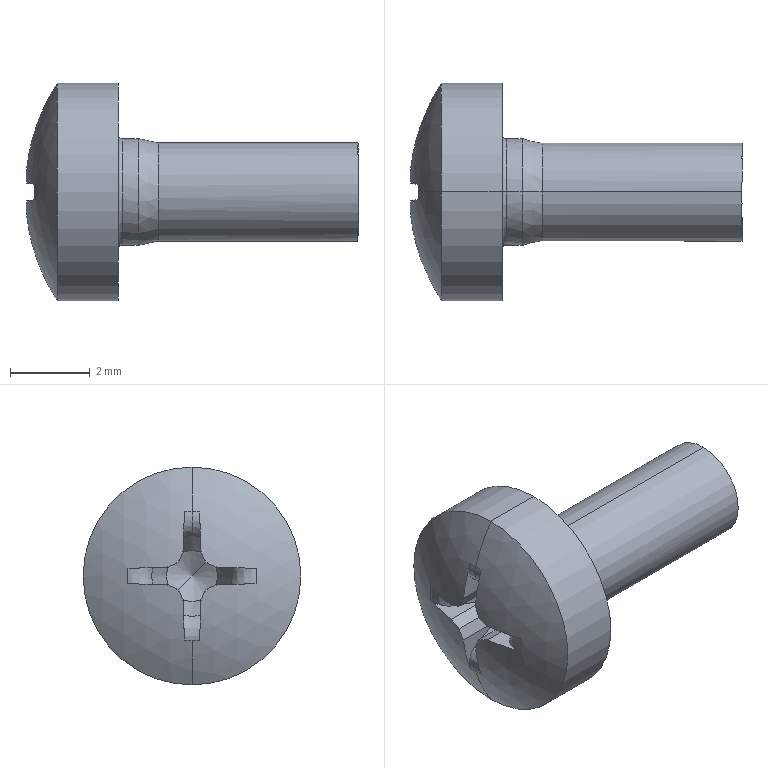Part | STEP file | 4-20.sldasm-Part-212 | 1 solid | 41 faces | box 8.306 x 5.45 x 5.45 mm | volume 72.235 mm3 | plane 18 | cone 8 | torus 7 | cylinder 6 | sphere 2 | commonest cylinder face diameters 2.458 x2 2.675 x2 5.45 x2
STEP:
#1=CARTESIAN_POINT('',(184.475,545.075,-91.754));
#2=VERTEX_POINT('',#1);
#3=CARTESIAN_POINT('',(184.475,545.075,-89.296));
#4=VERTEX_POINT('',#3);
#5=CARTESIAN_POINT('',(184.475,545.075,-90.525));
#6=DIRECTION('',(-1.,0.,0.));
#7=DIRECTION('',(0.,0.,1.));
#8=AXIS2_PLACEMENT_3D('',#5,#6,#7);
#9=CIRCLE('',#8,1.229);
#10=EDGE_CURVE('',#2,#4,#9,.T.);
#11=ORIENTED_EDGE('',*,*,#10,.T.);
#12=CARTESIAN_POINT('',(183.975,545.075,-89.188));
#13=VERTEX_POINT('',#12);
#14=CARTESIAN_POINT('',(184.475,545.075,-89.296));
#15=DIRECTION('',(-0.9776,0.,0.2107));
#16=VECTOR('',#15,1000.);
#17=LINE('',#14,#16);
#18=EDGE_CURVE('',#4,#13,#17,.T.);
#19=ORIENTED_EDGE('',*,*,#18,.T.);
#20=CARTESIAN_POINT('',(183.975,545.075,-91.862));
#21=VERTEX_POINT('',#20);
#22=CARTESIAN_POINT('',(183.975,545.075,-91.862));
#23=CARTESIAN_POINT('',(183.975,544.9,-91.863));
#24=CARTESIAN_POINT('',(183.975,544.725,-91.828));
#25=CARTESIAN_POINT('',(183.975,544.401,-91.694));
#26=CARTESIAN_POINT('',(183.975,544.253,-91.595));
#27=CARTESIAN_POINT('',(183.975,544.005,-91.347));
#28=CARTESIAN_POINT('',(183.975,543.906,-91.199));
#29=CARTESIAN_POINT('',(183.975,543.772,-90.875));
#30=CARTESIAN_POINT('',(183.975,543.737,-90.7));
#31=CARTESIAN_POINT('',(183.975,543.737,-90.35));
#32=CARTESIAN_POINT('',(183.975,543.772,-90.175));
#33=CARTESIAN_POINT('',(183.975,543.906,-89.851));
#34=CARTESIAN_POINT('',(183.975,544.005,-89.703));
#35=CARTESIAN_POINT('',(183.975,544.253,-89.455));
#36=CARTESIAN_POINT('',(183.975,544.401,-89.356));
#37=CARTESIAN_POINT('',(183.975,544.725,-89.222));
#38=CARTESIAN_POINT('',(183.975,544.9,-89.187));
#39=CARTESIAN_POINT('',(183.975,545.075,-89.188));
#40=B_SPLINE_CURVE_WITH_KNOTS('',3,(#22,#23,#24,#25,#26,#27,#28,#29,#30,#31,#32,#33,#34,#35,#36,#37,#38,#39),.UNSPECIFIED.,.F.,.F.,(4,2,2,2,2,2,2,2,4),(0.5,0.5625,0.625,0.6875,0.75,0.8125,0.875,0.9375,1.),.UNSPECIFIED.);
#41=EDGE_CURVE('',#21,#13,#40,.T.);
#42=ORIENTED_EDGE('',*,*,#41,.F.);
#43=CARTESIAN_POINT('',(184.475,545.075,-91.754));
#44=DIRECTION('',(-0.9776,0.,-0.2107));
#45=VECTOR('',#44,1000.);
#46=LINE('',#43,#45);
#47=EDGE_CURVE('',#2,#21,#46,.T.);
#48=ORIENTED_EDGE('',*,*,#47,.F.);
#49=EDGE_LOOP('',(#11,#19,#42,#48));
#50=FACE_OUTER_BOUND('',#49,.T.);
#51=CARTESIAN_POINT('',(184.475,545.075,-90.525));
#52=DIRECTION('',(-1.,0.,0.));
#53=DIRECTION('',(0.,0.,-1.));
#54=AXIS2_PLACEMENT_3D('',#51,#52,#53);
#55=CONICAL_SURFACE('',#54,1.229,0.2123);
#56=ADVANCED_FACE('',(#50),#55,.T.);
#57=ORIENTED_EDGE('',*,*,#10,.F.);
#58=CARTESIAN_POINT('',(189.475,545.075,-91.754));
#59=VERTEX_POINT('',#58);
#60=CARTESIAN_POINT('',(184.475,545.075,-91.754));
#61=DIRECTION('',(1.,0.,0.));
#62=VECTOR('',#61,1000.);
#63=LINE('',#60,#62);
#64=EDGE_CURVE('',#2,#59,#63,.T.);
#65=ORIENTED_EDGE('',*,*,#64,.T.);
#66=CARTESIAN_POINT('',(189.475,545.075,-89.296));
#67=VERTEX_POINT('',#66);
#68=CARTESIAN_POINT('',(189.475,545.075,-89.296));
#69=CARTESIAN_POINT('',(189.475,544.912,-89.296));
#70=CARTESIAN_POINT('',(189.475,544.756,-89.327));
#71=CARTESIAN_POINT('',(189.475,544.529,-89.421));
#72=CARTESIAN_POINT('',(189.475,544.423,-89.478));
#73=CARTESIAN_POINT('',(189.475,544.327,-89.549));
#74=CARTESIAN_POINT('',(189.475,544.265,-89.6));
#75=CARTESIAN_POINT('',(189.475,544.236,-89.626));
#76=CARTESIAN_POINT('',(189.475,543.966,-89.897));
#77=CARTESIAN_POINT('',(189.475,543.846,-90.185));
#78=CARTESIAN_POINT('',(189.475,543.846,-90.865));
#79=CARTESIAN_POINT('',(189.475,543.966,-91.154));
#80=CARTESIAN_POINT('',(189.475,544.447,-91.634));
#81=CARTESIAN_POINT('',(189.475,544.735,-91.754));
#82=CARTESIAN_POINT('',(189.475,545.075,-91.754));
#83=B_SPLINE_CURVE_WITH_KNOTS('',3,(#68,#69,#70,#71,#72,#73,#74,#75,#76,#77,#78,#79,#80,#81,#82),.UNSPECIFIED.,.F.,.F.,(4,2,1,2,2,2,2,4),(0.,0.0625,0.09375,0.1094,0.125,0.25,0.375,0.5),.UNSPECIFIED.);
#84=EDGE_CURVE('',#67,#59,#83,.T.);
#85=ORIENTED_EDGE('',*,*,#84,.F.);
#86=CARTESIAN_POINT('',(184.475,545.075,-89.296));
#87=DIRECTION('',(1.,0.,0.));
#88=VECTOR('',#87,1000.);
#89=LINE('',#86,#88);
#90=EDGE_CURVE('',#4,#67,#89,.T.);
#91=ORIENTED_EDGE('',*,*,#90,.F.);
#92=EDGE_LOOP('',(#57,#65,#85,#91));
#93=FACE_OUTER_BOUND('',#92,.T.);
#94=CARTESIAN_POINT('',(184.475,545.075,-90.525));
#95=DIRECTION('',(1.,0.,0.));
#96=DIRECTION('',(0.,0.,1.));
#97=AXIS2_PLACEMENT_3D('',#94,#95,#96);
#98=CYLINDRICAL_SURFACE('',#97,1.229);
#99=ADVANCED_FACE('',(#93),#98,.T.);
#100=CARTESIAN_POINT('',(181.663,545.281,-89.541));
#101=VERTEX_POINT('',#100);
#102=CARTESIAN_POINT('',(181.663,545.075,-89.52));
#103=VERTEX_POINT('',#102);
#104=CARTESIAN_POINT('',(181.663,545.075,-90.525));
#105=DIRECTION('',(1.,0.,0.));
#106=DIRECTION('',(0.,0.,-1.));
#107=AXIS2_PLACEMENT_3D('',#104,#105,#106);
#108=CIRCLE('',#107,1.005);
#109=EDGE_CURVE('',#101,#103,#108,.T.);
#110=ORIENTED_EDGE('',*,*,#109,.T.);
#111=CARTESIAN_POINT('',(181.413,545.075,-88.911));
#112=VERTEX_POINT('',#111);
#113=CARTESIAN_POINT('',(181.886,545.075,-89.072));
#114=DIRECTION('',(0.,1.,0.));
#115=DIRECTION('',(0.,0.,1.));
#116=AXIS2_PLACEMENT_3D('',#113,#114,#115);
#117=CIRCLE('',#116,0.5);
#118=EDGE_CURVE('',#103,#112,#117,.T.);
#119=ORIENTED_EDGE('',*,*,#118,.T.);
#120=CARTESIAN_POINT('',(181.413,545.27,-88.923));
#121=VERTEX_POINT('',#120);
#122=CARTESIAN_POINT('',(181.413,545.075,-90.525));
#123=DIRECTION('',(-1.,0.,0.));
#124=DIRECTION('',(0.,0.,1.));
#125=AXIS2_PLACEMENT_3D('',#122,#123,#124);
#126=CIRCLE('',#125,1.614);
#127=EDGE_CURVE('',#112,#121,#126,.T.);
#128=ORIENTED_EDGE('',*,*,#127,.T.);
#129=CARTESIAN_POINT('',(181.413,545.27,-88.923));
#130=CARTESIAN_POINT('',(181.374,545.272,-89.039));
#131=CARTESIAN_POINT('',(181.378,545.274,-89.166));
#132=CARTESIAN_POINT('',(181.469,545.278,-89.391));
#133=CARTESIAN_POINT('',(181.554,545.28,-89.486));
#134=CARTESIAN_POINT('',(181.663,545.281,-89.541));
#135=B_SPLINE_CURVE_WITH_KNOTS('',3,(#129,#130,#131,#132,#133,#134),.UNSPECIFIED.,.F.,.F.,(4,2,4),(0.,0.0003614,0.0007228),.UNSPECIFIED.);
#136=EDGE_CURVE('',#121,#101,#135,.T.);
#137=ORIENTED_EDGE('',*,*,#136,.T.);
#138=EDGE_LOOP('',(#110,#119,#128,#137));
#139=FACE_OUTER_BOUND('',#138,.T.);
#140=CARTESIAN_POINT('',(181.886,545.075,-90.525));
#141=DIRECTION('',(1.,0.,0.));
#142=DIRECTION('',(0.,0.,1.));
#143=AXIS2_PLACEMENT_3D('',#140,#141,#142);
#144=TOROIDAL_SURFACE('',#143,1.453,0.5);
#145=ADVANCED_FACE('',(#139),#144,.T.);
#146=CARTESIAN_POINT('',(182.745,545.075,-90.525));
#147=VERTEX_POINT('',#146);
#148=CARTESIAN_POINT('',(182.485,545.418,-90.868));
#149=VERTEX_POINT('',#148);
#150=CARTESIAN_POINT('',(182.745,545.075,-90.525));
#151=DIRECTION('',(-0.472,0.6234,-0.6234));
#152=VECTOR('',#151,1000.);
#153=LINE('',#150,#152);
#154=EDGE_CURVE('',#147,#149,#153,.T.);
#155=ORIENTED_EDGE('',*,*,#154,.F.);
#156=CARTESIAN_POINT('',(182.485,544.732,-90.182));
#157=VERTEX_POINT('',#156);
#158=CARTESIAN_POINT('',(182.745,545.075,-90.525));
#159=DIRECTION('',(-0.472,-0.6234,0.6234));
#160=VECTOR('',#159,1000.);
#161=LINE('',#158,#160);
#162=EDGE_CURVE('',#147,#157,#161,.T.);
#163=ORIENTED_EDGE('',*,*,#162,.T.);
#164=CARTESIAN_POINT('',(182.405,544.842,-89.934));
#165=VERTEX_POINT('',#164);
#166=CARTESIAN_POINT('',(182.485,544.732,-90.182));
#167=CARTESIAN_POINT('',(182.467,544.77,-90.097));
#168=CARTESIAN_POINT('',(182.438,544.806,-90.015));
#169=CARTESIAN_POINT('',(182.405,544.842,-89.934));
#170=B_SPLINE_CURVE_WITH_KNOTS('',3,(#166,#167,#168,#169),.UNSPECIFIED.,.F.,.F.,(4,4),(0.000000222,0.0002833),.UNSPECIFIED.);
#171=EDGE_CURVE('',#157,#165,#170,.T.);
#172=ORIENTED_EDGE('',*,*,#171,.T.);
#173=CARTESIAN_POINT('',(182.405,545.308,-89.934));
#174=VERTEX_POINT('',#173);
#175=CARTESIAN_POINT('',(182.405,545.075,-90.525));
#176=DIRECTION('',(-1.,0.,0.));
#177=DIRECTION('',(0.,-0.7071,0.7071));
#178=AXIS2_PLACEMENT_3D('',#175,#176,#177);
#179=CIRCLE('',#178,0.635);
#180=EDGE_CURVE('',#165,#174,#179,.T.);
#181=ORIENTED_EDGE('',*,*,#180,.T.);
#182=CARTESIAN_POINT('',(182.485,545.418,-90.182));
#183=VERTEX_POINT('',#182);
#184=CARTESIAN_POINT('',(182.405,545.308,-89.934));
#185=CARTESIAN_POINT('',(182.438,545.344,-90.015));
#186=CARTESIAN_POINT('',(182.467,545.38,-90.097));
#187=CARTESIAN_POINT('',(182.485,545.418,-90.182));
#188=B_SPLINE_CURVE_WITH_KNOTS('',3,(#184,#185,#186,#187),.UNSPECIFIED.,.F.,.F.,(4,4),(0.000000567,0.0002836),.UNSPECIFIED.);
#189=EDGE_CURVE('',#174,#183,#188,.T.);
#190=ORIENTED_EDGE('',*,*,#189,.T.);
#191=CARTESIAN_POINT('',(182.405,545.666,-90.292));
#192=VERTEX_POINT('',#191);
#193=CARTESIAN_POINT('',(182.485,545.418,-90.182));
#194=CARTESIAN_POINT('',(182.467,545.503,-90.22));
#195=CARTESIAN_POINT('',(182.438,545.585,-90.256));
#196=CARTESIAN_POINT('',(182.405,545.666,-90.292));
#197=B_SPLINE_CURVE_WITH_KNOTS('',3,(#193,#194,#195,#196),.UNSPECIFIED.,.F.,.F.,(4,4),(0.000000222,0.0002833),.UNSPECIFIED.);
#198=EDGE_CURVE('',#183,#192,#197,.T.);
#199=ORIENTED_EDGE('',*,*,#198,.T.);
#200=CARTESIAN_POINT('',(182.405,545.666,-90.758));
#201=VERTEX_POINT('',#200);
#202=CARTESIAN_POINT('',(182.405,545.075,-90.525));
#203=DIRECTION('',(-1.,0.,0.));
#204=DIRECTION('',(0.,-0.7071,0.7071));
#205=AXIS2_PLACEMENT_3D('',#202,#203,#204);
#206=CIRCLE('',#205,0.635);
#207=EDGE_CURVE('',#192,#201,#206,.T.);
#208=ORIENTED_EDGE('',*,*,#207,.T.);
#209=CARTESIAN_POINT('',(182.405,545.666,-90.758));
#210=CARTESIAN_POINT('',(182.438,545.585,-90.794));
#211=CARTESIAN_POINT('',(182.467,545.503,-90.83));
#212=CARTESIAN_POINT('',(182.485,545.418,-90.868));
#213=B_SPLINE_CURVE_WITH_KNOTS('',3,(#209,#210,#211,#212),.UNSPECIFIED.,.F.,.F.,(4,4),(0.000000567,0.0002836),.UNSPECIFIED.);
#214=EDGE_CURVE('',#201,#149,#213,.T.);
#215=ORIENTED_EDGE('',*,*,#214,.T.);
#216=EDGE_LOOP('',(#155,#163,#172,#181,#190,#199,#208,#215));
#217=FACE_OUTER_BOUND('',#216,.T.);
#218=CARTESIAN_POINT('',(-817.255,545.075,-90.525));
#219=DIRECTION('',(-1.,0.,0.));
#220=DIRECTION('',(0.,0.7071,-0.7071));
#221=AXIS2_PLACEMENT_3D('',#218,#219,#220);
#222=CONICAL_SURFACE('',#221,1867.647,1.079);
#223=ADVANCED_FACE('',(#217),#222,.F.);
#224=CARTESIAN_POINT('',(183.575,545.075,-89.187));
#225=VERTEX_POINT('',#224);
#226=CARTESIAN_POINT('',(183.575,545.075,-91.863));
#227=VERTEX_POINT('',#226);
#228=CARTESIAN_POINT('',(183.575,545.075,-90.525));
#229=DIRECTION('',(-1.,0.,0.));
#230=DIRECTION('',(0.,0.,1.));
#231=AXIS2_PLACEMENT_3D('',#228,#229,#230);
#232=CIRCLE('',#231,1.338);
#233=EDGE_CURVE('',#225,#227,#232,.T.);
#234=ORIENTED_EDGE('',*,*,#233,.T.);
#235=CARTESIAN_POINT('',(183.475,545.075,-91.963));
#236=VERTEX_POINT('',#235);
#237=CARTESIAN_POINT('',(183.575,545.075,-91.963));
#238=DIRECTION('',(0.,-1.,0.));
#239=DIRECTION('',(0.,0.,-1.));
#240=AXIS2_PLACEMENT_3D('',#237,#238,#239);
#241=CIRCLE('',#240,0.1);
#242=EDGE_CURVE('',#227,#236,#241,.T.);
#243=ORIENTED_EDGE('',*,*,#242,.T.);
#244=CARTESIAN_POINT('',(183.475,545.075,-89.087));
#245=VERTEX_POINT('',#244);
#246=CARTESIAN_POINT('',(183.475,545.075,-90.525));
#247=DIRECTION('',(1.,0.,0.));
#248=DIRECTION('',(0.,0.,1.));
#249=AXIS2_PLACEMENT_3D('',#246,#247,#248);
#250=CIRCLE('',#249,1.438);
#251=EDGE_CURVE('',#236,#245,#250,.T.);
#252=ORIENTED_EDGE('',*,*,#251,.T.);
#253=CARTESIAN_POINT('',(183.575,545.075,-89.087));
#254=DIRECTION('',(0.,1.,0.));
#255=DIRECTION('',(0.,0.,1.));
#256=AXIS2_PLACEMENT_3D('',#253,#254,#255);
#257=CIRCLE('',#256,0.1);
#258=EDGE_CURVE('',#225,#245,#257,.T.);
#259=ORIENTED_EDGE('',*,*,#258,.F.);
#260=EDGE_LOOP('',(#234,#243,#252,#259));
#261=FACE_OUTER_BOUND('',#260,.T.);
#262=CARTESIAN_POINT('',(183.575,545.075,-90.525));
#263=DIRECTION('',(1.,0.,0.));
#264=DIRECTION('',(0.,0.,1.));
#265=AXIS2_PLACEMENT_3D('',#262,#263,#264);
#266=TOROIDAL_SURFACE('',#265,1.438,0.1);
#267=ADVANCED_FACE('',(#261),#266,.F.);
#268=CARTESIAN_POINT('',(183.575,545.075,-90.525));
#269=DIRECTION('',(-1.,0.,0.));
#270=DIRECTION('',(0.,0.,1.));
#271=AXIS2_PLACEMENT_3D('',#268,#269,#270);
#272=CIRCLE('',#271,1.338);
#273=EDGE_CURVE('',#227,#225,#272,.T.);
#274=ORIENTED_EDGE('',*,*,#273,.F.);
#275=CARTESIAN_POINT('',(183.475,545.075,-91.863));
#276=DIRECTION('',(1.,0.,0.));
#277=VECTOR('',#276,1000.);
#278=LINE('',#275,#277);
#279=EDGE_CURVE('',#227,#21,#278,.T.);
#280=ORIENTED_EDGE('',*,*,#279,.T.);
#281=ORIENTED_EDGE('',*,*,#41,.T.);
#282=CARTESIAN_POINT('',(183.475,545.075,-89.187));
#283=DIRECTION('',(1.,0.,0.));
#284=VECTOR('',#283,1000.);
#285=LINE('',#282,#284);
#286=EDGE_CURVE('',#225,#13,#285,.T.);
#287=ORIENTED_EDGE('',*,*,#286,.F.);
#288=EDGE_LOOP('',(#274,#280,#281,#287));
#289=FACE_OUTER_BOUND('',#288,.T.);
#290=CARTESIAN_POINT('',(183.475,545.075,-90.525));
#291=DIRECTION('',(1.,0.,0.));
#292=DIRECTION('',(0.,0.,1.));
#293=AXIS2_PLACEMENT_3D('',#290,#291,#292);
#294=CYLINDRICAL_SURFACE('',#293,1.338);
#295=ADVANCED_FACE('',(#289),#294,.T.);
#296=CARTESIAN_POINT('',(181.953,545.075,-87.8));
#297=VERTEX_POINT('',#296);
#298=CARTESIAN_POINT('',(181.953,545.075,-93.25));
#299=VERTEX_POINT('',#298);
#300=CARTESIAN_POINT('',(181.953,545.075,-90.525));
#301=DIRECTION('',(1.,0.,0.));
#302=DIRECTION('',(0.,0.,1.));
#303=AXIS2_PLACEMENT_3D('',#300,#301,#302);
#304=CIRCLE('',#303,2.725);
#305=EDGE_CURVE('',#297,#299,#304,.T.);
#306=ORIENTED_EDGE('',*,*,#305,.F.);
#307=CARTESIAN_POINT('',(186.145,545.075,-90.525));
#308=DIRECTION('',(0.,-1.,0.));
#309=DIRECTION('',(0.,0.,-1.));
#310=AXIS2_PLACEMENT_3D('',#307,#308,#309);
#311=CIRCLE('',#310,5.);
#312=EDGE_CURVE('',#297,#112,#311,.T.);
#313=ORIENTED_EDGE('',*,*,#312,.T.);
#314=CARTESIAN_POINT('',(181.413,544.88,-88.923));
#315=VERTEX_POINT('',#314);
#316=CARTESIAN_POINT('',(181.413,545.075,-90.525));
#317=DIRECTION('',(-1.,0.,0.));
#318=DIRECTION('',(0.,0.,1.));
#319=AXIS2_PLACEMENT_3D('',#316,#317,#318);
#320=CIRCLE('',#319,1.614);
#321=EDGE_CURVE('',#315,#112,#320,.T.);
#322=ORIENTED_EDGE('',*,*,#321,.F.);
#323=CARTESIAN_POINT('',(181.19,544.863,-89.888));
#324=VERTEX_POINT('',#323);
#325=CARTESIAN_POINT('',(186.145,544.852,-90.521));
#326=DIRECTION('',(0.,-0.9998,0.01745));
#327=DIRECTION('',(0.,-0.01745,-0.9998));
#328=AXIS2_PLACEMENT_3D('',#325,#326,#327);
#329=CIRCLE('',#328,4.995);
#330=EDGE_CURVE('',#315,#324,#329,.T.);
#331=ORIENTED_EDGE('',*,*,#330,.T.);
#332=CARTESIAN_POINT('',(181.169,544.732,-90.182));
#333=VERTEX_POINT('',#332);
#334=CARTESIAN_POINT('',(186.145,544.661,-90.341));
#335=DIRECTION('',(0.,-0.9135,0.4067));
#336=DIRECTION('',(0.,-0.4067,-0.9135));
#337=AXIS2_PLACEMENT_3D('',#334,#335,#336);
#338=CIRCLE('',#337,4.979);
#339=EDGE_CURVE('',#324,#333,#338,.T.);
#340=ORIENTED_EDGE('',*,*,#339,.T.);
#341=CARTESIAN_POINT('',(181.19,544.438,-90.313));
#342=VERTEX_POINT('',#341);
#343=CARTESIAN_POINT('',(186.145,544.891,-90.111));
#344=DIRECTION('',(0.,-0.4067,0.9135));
#345=DIRECTION('',(0.,-0.9135,-0.4067));
#346=AXIS2_PLACEMENT_3D('',#343,#344,#345);
#347=CIRCLE('',#346,4.979);
#348=EDGE_CURVE('',#333,#342,#347,.T.);
#349=ORIENTED_EDGE('',*,*,#348,.T.);
#350=CARTESIAN_POINT('',(181.413,543.473,-90.33));
#351=VERTEX_POINT('',#350);
#352=CARTESIAN_POINT('',(186.145,545.071,-90.302));
#353=DIRECTION('',(0.,-0.01745,0.9998));
#354=DIRECTION('',(0.,-0.9998,-0.01745));
#355=AXIS2_PLACEMENT_3D('',#352,#353,#354);
#356=CIRCLE('',#355,4.995);
#357=EDGE_CURVE('',#342,#351,#356,.T.);
#358=ORIENTED_EDGE('',*,*,#357,.T.);
#359=CARTESIAN_POINT('',(181.413,543.473,-90.72));
#360=VERTEX_POINT('',#359);
#361=CARTESIAN_POINT('',(181.413,545.075,-90.525));
#362=DIRECTION('',(-1.,0.,0.));
#363=DIRECTION('',(0.,0.,1.));
#364=AXIS2_PLACEMENT_3D('',#361,#362,#363);
#365=CIRCLE('',#364,1.614);
#366=EDGE_CURVE('',#360,#351,#365,.T.);
#367=ORIENTED_EDGE('',*,*,#366,.F.);
#368=CARTESIAN_POINT('',(181.19,544.438,-90.737));
#369=VERTEX_POINT('',#368);
#370=CARTESIAN_POINT('',(186.145,545.071,-90.748));
#371=DIRECTION('',(0.,-0.01745,-0.9998));
#372=DIRECTION('',(0.,0.9998,-0.01745));
#373=AXIS2_PLACEMENT_3D('',#370,#371,#372);
#374=CIRCLE('',#373,4.995);
#375=EDGE_CURVE('',#360,#369,#374,.T.);
#376=ORIENTED_EDGE('',*,*,#375,.T.);
#377=CARTESIAN_POINT('',(181.169,544.732,-90.868));
#378=VERTEX_POINT('',#377);
#379=CARTESIAN_POINT('',(186.145,544.891,-90.939));
#380=DIRECTION('',(0.,-0.4067,-0.9135));
#381=DIRECTION('',(0.,0.9135,-0.4067));
#382=AXIS2_PLACEMENT_3D('',#379,#380,#381);
#383=CIRCLE('',#382,4.979);
#384=EDGE_CURVE('',#369,#378,#383,.T.);
#385=ORIENTED_EDGE('',*,*,#384,.T.);
#386=CARTESIAN_POINT('',(181.19,544.863,-91.162));
#387=VERTEX_POINT('',#386);
#388=CARTESIAN_POINT('',(186.145,544.661,-90.709));
#389=DIRECTION('',(0.,-0.9135,-0.4067));
#390=DIRECTION('',(0.,0.4067,-0.9135));
#391=AXIS2_PLACEMENT_3D('',#388,#389,#390);
#392=CIRCLE('',#391,4.979);
#393=EDGE_CURVE('',#378,#387,#392,.T.);
#394=ORIENTED_EDGE('',*,*,#393,.T.);
#395=CARTESIAN_POINT('',(181.413,544.88,-92.127));
#396=VERTEX_POINT('',#395);
#397=CARTESIAN_POINT('',(186.145,544.852,-90.529));
#398=DIRECTION('',(0.,-0.9998,-0.01745));
#399=DIRECTION('',(0.,0.01745,-0.9998));
#400=AXIS2_PLACEMENT_3D('',#397,#398,#399);
#401=CIRCLE('',#400,4.995);
#402=EDGE_CURVE('',#387,#396,#401,.T.);
#403=ORIENTED_EDGE('',*,*,#402,.T.);
#404=CARTESIAN_POINT('',(181.413,545.075,-92.139));
#405=VERTEX_POINT('',#404);
#406=CARTESIAN_POINT('',(181.413,545.075,-90.525));
#407=DIRECTION('',(-1.,0.,0.));
#408=DIRECTION('',(0.,0.,1.));
#409=AXIS2_PLACEMENT_3D('',#406,#407,#408);
#410=CIRCLE('',#409,1.614);
#411=EDGE_CURVE('',#405,#396,#410,.T.);
#412=ORIENTED_EDGE('',*,*,#411,.F.);
#413=CARTESIAN_POINT('',(186.145,545.075,-90.525));
#414=DIRECTION('',(0.,1.,0.));
#415=DIRECTION('',(0.,0.,1.));
#416=AXIS2_PLACEMENT_3D('',#413,#414,#415);
#417=CIRCLE('',#416,5.);
#418=EDGE_CURVE('',#299,#405,#417,.T.);
#419=ORIENTED_EDGE('',*,*,#418,.F.);
#420=EDGE_LOOP('',(#306,#313,#322,#331,#340,#349,#358,#367,#376,#385,#394,#403,#412,#419));
#421=FACE_OUTER_BOUND('',#420,.T.);
#422=CARTESIAN_POINT('',(186.145,545.075,-90.525));
#423=DIRECTION('',(0.,-1.,0.));
#424=DIRECTION('',(0.,0.,-1.));
#425=AXIS2_PLACEMENT_3D('',#422,#423,#424);
#426=SPHERICAL_SURFACE('',#425,5.);
#427=ADVANCED_FACE('',(#421),#426,.T.);
#428=ORIENTED_EDGE('',*,*,#305,.T.);
#429=CARTESIAN_POINT('',(183.475,545.075,-93.25));
#430=VERTEX_POINT('',#429);
#431=CARTESIAN_POINT('',(181.145,545.075,-93.25));
#432=DIRECTION('',(1.,0.,0.));
#433=VECTOR('',#432,1000.);
#434=LINE('',#431,#433);
#435=EDGE_CURVE('',#299,#430,#434,.T.);
#436=ORIENTED_EDGE('',*,*,#435,.T.);
#437=CARTESIAN_POINT('',(183.475,545.075,-87.8));
#438=VERTEX_POINT('',#437);
#439=CARTESIAN_POINT('',(183.475,545.075,-90.525));
#440=DIRECTION('',(1.,0.,0.));
#441=DIRECTION('',(0.,0.,-1.));
#442=AXIS2_PLACEMENT_3D('',#439,#440,#441);
#443=CIRCLE('',#442,2.725);
#444=EDGE_CURVE('',#438,#430,#443,.T.);
#445=ORIENTED_EDGE('',*,*,#444,.F.);
#446=CARTESIAN_POINT('',(181.145,545.075,-87.8));
#447=DIRECTION('',(1.,0.,0.));
#448=VECTOR('',#447,1000.);
#449=LINE('',#446,#448);
#450=EDGE_CURVE('',#297,#438,#449,.T.);
#451=ORIENTED_EDGE('',*,*,#450,.F.);
#452=EDGE_LOOP('',(#428,#436,#445,#451));
#453=FACE_OUTER_BOUND('',#452,.T.);
#454=CARTESIAN_POINT('',(181.145,545.075,-90.525));
#455=DIRECTION('',(1.,0.,0.));
#456=DIRECTION('',(0.,0.,1.));
#457=AXIS2_PLACEMENT_3D('',#454,#455,#456);
#458=CYLINDRICAL_SURFACE('',#457,2.725);
#459=ADVANCED_FACE('',(#453),#458,.T.);
#460=CARTESIAN_POINT('',(183.475,545.075,-90.525));
#461=DIRECTION('',(1.,0.,0.));
#462=DIRECTION('',(0.,0.,1.));
#463=AXIS2_PLACEMENT_3D('',#460,#461,#462);
#464=CIRCLE('',#463,1.438);
#465=EDGE_CURVE('',#245,#236,#464,.T.);
#466=ORIENTED_EDGE('',*,*,#465,.F.);
#467=ORIENTED_EDGE('',*,*,#251,.F.);
#468=EDGE_LOOP('',(#466,#467));
#469=FACE_BOUND('',#468,.T.);
#470=ORIENTED_EDGE('',*,*,#444,.T.);
#471=CARTESIAN_POINT('',(183.475,545.075,-90.525));
#472=DIRECTION('',(1.,0.,0.));
#473=DIRECTION('',(0.,0.,-1.));
#474=AXIS2_PLACEMENT_3D('',#471,#472,#473);
#475=CIRCLE('',#474,2.725);
#476=EDGE_CURVE('',#430,#438,#475,.T.);
#477=ORIENTED_EDGE('',*,*,#476,.T.);
#478=EDGE_LOOP('',(#470,#477));
#479=FACE_OUTER_BOUND('',#478,.T.);
#480=CARTESIAN_POINT('',(183.475,545.075,-90.525));
#481=DIRECTION('',(1.,0.,0.));
#482=DIRECTION('',(0.,0.,1.));
#483=AXIS2_PLACEMENT_3D('',#480,#481,#482);
#484=PLANE('',#483);
#485=ADVANCED_FACE('',(#469,#479),#484,.T.);
#486=ORIENTED_EDGE('',*,*,#435,.F.);
#487=CARTESIAN_POINT('',(181.953,545.075,-90.525));
#488=DIRECTION('',(1.,0.,0.));
#489=DIRECTION('',(0.,0.,1.));
#490=AXIS2_PLACEMENT_3D('',#487,#488,#489);
#491=CIRCLE('',#490,2.725);
#492=EDGE_CURVE('',#299,#297,#491,.T.);
#493=ORIENTED_EDGE('',*,*,#492,.T.);
#494=ORIENTED_EDGE('',*,*,#450,.T.);
#495=ORIENTED_EDGE('',*,*,#476,.F.);
#496=EDGE_LOOP('',(#486,#493,#494,#495));
#497=FACE_OUTER_BOUND('',#496,.T.);
#498=CARTESIAN_POINT('',(181.145,545.075,-90.525));
#499=DIRECTION('',(1.,0.,0.));
#500=DIRECTION('',(0.,0.,1.));
#501=AXIS2_PLACEMENT_3D('',#498,#499,#500);
#502=CYLINDRICAL_SURFACE('',#501,2.725);
#503=ADVANCED_FACE('',(#497),#502,.T.);
#504=ORIENTED_EDGE('',*,*,#312,.F.);
#505=ORIENTED_EDGE('',*,*,#492,.F.);
#506=ORIENTED_EDGE('',*,*,#418,.T.);
#507=CARTESIAN_POINT('',(181.413,545.27,-92.127));
#508=VERTEX_POINT('',#507);
#509=CARTESIAN_POINT('',(181.413,545.075,-90.525));
#510=DIRECTION('',(-1.,0.,0.));
#511=DIRECTION('',(0.,0.,1.));
#512=AXIS2_PLACEMENT_3D('',#509,#510,#511);
#513=CIRCLE('',#512,1.614);
#514=EDGE_CURVE('',#508,#405,#513,.T.);
#515=ORIENTED_EDGE('',*,*,#514,.F.);
#516=CARTESIAN_POINT('',(181.19,545.287,-91.162));
#517=VERTEX_POINT('',#516);
#518=CARTESIAN_POINT('',(186.145,545.298,-90.529));
#519=DIRECTION('',(0.,0.9998,-0.01745));
#520=DIRECTION('',(0.,0.01745,0.9998));
#521=AXIS2_PLACEMENT_3D('',#518,#519,#520);
#522=CIRCLE('',#521,4.995);
#523=EDGE_CURVE('',#508,#517,#522,.T.);
#524=ORIENTED_EDGE('',*,*,#523,.T.);
#525=CARTESIAN_POINT('',(181.169,545.418,-90.868));
#526=VERTEX_POINT('',#525);
#527=CARTESIAN_POINT('',(186.145,545.489,-90.709));
#528=DIRECTION('',(0.,0.9135,-0.4067));
#529=DIRECTION('',(0.,0.4067,0.9135));
#530=AXIS2_PLACEMENT_3D('',#527,#528,#529);
#531=CIRCLE('',#530,4.979);
#532=EDGE_CURVE('',#517,#526,#531,.T.);
#533=ORIENTED_EDGE('',*,*,#532,.T.);
#534=CARTESIAN_POINT('',(181.19,545.712,-90.737));
#535=VERTEX_POINT('',#534);
#536=CARTESIAN_POINT('',(186.145,545.259,-90.939));
#537=DIRECTION('',(0.,0.4067,-0.9135));
#538=DIRECTION('',(0.,0.9135,0.4067));
#539=AXIS2_PLACEMENT_3D('',#536,#537,#538);
#540=CIRCLE('',#539,4.979);
#541=EDGE_CURVE('',#526,#535,#540,.T.);
#542=ORIENTED_EDGE('',*,*,#541,.T.);
#543=CARTESIAN_POINT('',(181.413,546.677,-90.72));
#544=VERTEX_POINT('',#543);
#545=CARTESIAN_POINT('',(186.145,545.079,-90.748));
#546=DIRECTION('',(0.,0.01745,-0.9998));
#547=DIRECTION('',(0.,0.9998,0.01745));
#548=AXIS2_PLACEMENT_3D('',#545,#546,#547);
#549=CIRCLE('',#548,4.995);
#550=EDGE_CURVE('',#535,#544,#549,.T.);
#551=ORIENTED_EDGE('',*,*,#550,.T.);
#552=CARTESIAN_POINT('',(181.413,546.677,-90.33));
#553=VERTEX_POINT('',#552);
#554=CARTESIAN_POINT('',(181.413,545.075,-90.525));
#555=DIRECTION('',(-1.,0.,0.));
#556=DIRECTION('',(0.,0.,1.));
#557=AXIS2_PLACEMENT_3D('',#554,#555,#556);
#558=CIRCLE('',#557,1.614);
#559=EDGE_CURVE('',#553,#544,#558,.T.);
#560=ORIENTED_EDGE('',*,*,#559,.F.);
#561=CARTESIAN_POINT('',(181.19,545.712,-90.313));
#562=VERTEX_POINT('',#561);
#563=CARTESIAN_POINT('',(186.145,545.079,-90.302));
#564=DIRECTION('',(0.,0.01745,0.9998));
#565=DIRECTION('',(0.,-0.9998,0.01745));
#566=AXIS2_PLACEMENT_3D('',#563,#564,#565);
#567=CIRCLE('',#566,4.995);
#568=EDGE_CURVE('',#553,#562,#567,.T.);
#569=ORIENTED_EDGE('',*,*,#568,.T.);
#570=CARTESIAN_POINT('',(181.169,545.418,-90.182));
#571=VERTEX_POINT('',#570);
#572=CARTESIAN_POINT('',(186.145,545.259,-90.111));
#573=DIRECTION('',(0.,0.4067,0.9135));
#574=DIRECTION('',(0.,-0.9135,0.4067));
#575=AXIS2_PLACEMENT_3D('',#572,#573,#574);
#576=CIRCLE('',#575,4.979);
#577=EDGE_CURVE('',#562,#571,#576,.T.);
#578=ORIENTED_EDGE('',*,*,#577,.T.);
#579=CARTESIAN_POINT('',(181.19,545.287,-89.888));
#580=VERTEX_POINT('',#579);
#581=CARTESIAN_POINT('',(186.145,545.489,-90.341));
#582=DIRECTION('',(0.,0.9135,0.4067));
#583=DIRECTION('',(0.,-0.4067,0.9135));
#584=AXIS2_PLACEMENT_3D('',#581,#582,#583);
#585=CIRCLE('',#584,4.979);
#586=EDGE_CURVE('',#571,#580,#585,.T.);
#587=ORIENTED_EDGE('',*,*,#586,.T.);
#588=CARTESIAN_POINT('',(186.145,545.298,-90.521));
#589=DIRECTION('',(0.,0.9998,0.01745));
#590=DIRECTION('',(0.,-0.01745,0.9998));
#591=AXIS2_PLACEMENT_3D('',#588,#589,#590);
#592=CIRCLE('',#591,4.995);
#593=EDGE_CURVE('',#580,#121,#592,.T.);
#594=ORIENTED_EDGE('',*,*,#593,.T.);
#595=ORIENTED_EDGE('',*,*,#127,.F.);
#596=EDGE_LOOP('',(#504,#505,#506,#515,#524,#533,#542,#551,#560,#569,#578,#587,#594,#595));
#597=FACE_OUTER_BOUND('',#596,.T.);
#598=CARTESIAN_POINT('',(186.145,545.075,-90.525));
#599=DIRECTION('',(0.,-1.,0.));
#600=DIRECTION('',(0.,0.,-1.));
#601=AXIS2_PLACEMENT_3D('',#598,#599,#600);
#602=SPHERICAL_SURFACE('',#601,5.);
#603=ADVANCED_FACE('',(#597),#602,.T.);
#604=ORIENTED_EDGE('',*,*,#279,.F.);
#605=ORIENTED_EDGE('',*,*,#233,.F.);
#606=ORIENTED_EDGE('',*,*,#286,.T.);
#607=CARTESIAN_POINT('',(183.975,545.075,-89.188));
#608=CARTESIAN_POINT('',(183.975,545.25,-89.187));
#609=CARTESIAN_POINT('',(183.975,545.425,-89.222));
#610=CARTESIAN_POINT('',(183.975,545.749,-89.356));
#611=CARTESIAN_POINT('',(183.975,545.897,-89.455));
#612=CARTESIAN_POINT('',(183.975,546.145,-89.703));
#613=CARTESIAN_POINT('',(183.975,546.244,-89.851));
#614=CARTESIAN_POINT('',(183.975,546.378,-90.175));
#615=CARTESIAN_POINT('',(183.975,546.413,-90.35));
#616=CARTESIAN_POINT('',(183.975,546.413,-90.7));
#617=CARTESIAN_POINT('',(183.975,546.378,-90.875));
#618=CARTESIAN_POINT('',(183.975,546.244,-91.199));
#619=CARTESIAN_POINT('',(183.975,546.145,-91.347));
#620=CARTESIAN_POINT('',(183.975,545.897,-91.595));
#621=CARTESIAN_POINT('',(183.975,545.749,-91.694));
#622=CARTESIAN_POINT('',(183.975,545.425,-91.828));
#623=CARTESIAN_POINT('',(183.975,545.25,-91.863));
#624=CARTESIAN_POINT('',(183.975,545.075,-91.862));
#625=B_SPLINE_CURVE_WITH_KNOTS('',3,(#607,#608,#609,#610,#611,#612,#613,#614,#615,#616,#617,#618,#619,#620,#621,#622,#623,#624),.UNSPECIFIED.,.F.,.F.,(4,2,2,2,2,2,2,2,4),(0.,0.0625,0.125,0.1875,0.25,0.3125,0.375,0.4375,0.5),.UNSPECIFIED.);
#626=EDGE_CURVE('',#13,#21,#625,.T.);
#627=ORIENTED_EDGE('',*,*,#626,.T.);
#628=EDGE_LOOP('',(#604,#605,#606,#627));
#629=FACE_OUTER_BOUND('',#628,.T.);
#630=CARTESIAN_POINT('',(183.475,545.075,-90.525));
#631=DIRECTION('',(1.,0.,0.));
#632=DIRECTION('',(0.,0.,1.));
#633=AXIS2_PLACEMENT_3D('',#630,#631,#632);
#634=CYLINDRICAL_SURFACE('',#633,1.338);
#635=ADVANCED_FACE('',(#629),#634,.T.);
#636=ORIENTED_EDGE('',*,*,#242,.F.);
#637=ORIENTED_EDGE('',*,*,#273,.T.);
#638=ORIENTED_EDGE('',*,*,#258,.T.);
#639=ORIENTED_EDGE('',*,*,#465,.T.);
#640=EDGE_LOOP('',(#636,#637,#638,#639));
#641=FACE_OUTER_BOUND('',#640,.T.);
#642=CARTESIAN_POINT('',(183.575,545.075,-90.525));
#643=DIRECTION('',(1.,0.,0.));
#644=DIRECTION('',(0.,0.,1.));
#645=AXIS2_PLACEMENT_3D('',#642,#643,#644);
#646=TOROIDAL_SURFACE('',#645,1.438,0.1);
#647=ADVANCED_FACE('',(#641),#646,.F.);
#648=CARTESIAN_POINT('',(181.663,544.869,-91.509));
#649=VERTEX_POINT('',#648);
#650=CARTESIAN_POINT('',(182.332,544.863,-91.162));
#651=VERTEX_POINT('',#650);
#652=CARTESIAN_POINT('',(181.663,544.869,-91.509));
#653=CARTESIAN_POINT('',(181.887,544.867,-91.394));
#654=CARTESIAN_POINT('',(182.11,544.865,-91.279));
#655=CARTESIAN_POINT('',(182.332,544.863,-91.162));
#656=B_SPLINE_CURVE_WITH_KNOTS('',3,(#652,#653,#654,#655),.UNSPECIFIED.,.F.,.F.,(4,4),(0.001527,0.002281),.UNSPECIFIED.);
#657=EDGE_CURVE('',#649,#651,#656,.T.);
#658=ORIENTED_EDGE('',*,*,#657,.T.);
#659=CARTESIAN_POINT('',(182.405,544.842,-91.116));
#660=VERTEX_POINT('',#659);
#661=CARTESIAN_POINT('',(182.332,544.863,-91.162));
#662=CARTESIAN_POINT('',(182.357,544.856,-91.147));
#663=CARTESIAN_POINT('',(182.381,544.849,-91.132));
#664=CARTESIAN_POINT('',(182.405,544.842,-91.116));
#665=B_SPLINE_CURVE_WITH_KNOTS('',3,(#661,#662,#663,#664),.UNSPECIFIED.,.F.,.F.,(4,4),(0.001734,0.001823),.UNSPECIFIED.);
#666=EDGE_CURVE('',#651,#660,#665,.T.);
#667=ORIENTED_EDGE('',*,*,#666,.T.);
#668=CARTESIAN_POINT('',(182.405,545.308,-91.116));
#669=VERTEX_POINT('',#668);
#670=CARTESIAN_POINT('',(182.405,545.075,-90.525));
#671=DIRECTION('',(-1.,0.,0.));
#672=DIRECTION('',(0.,-0.7071,0.7071));
#673=AXIS2_PLACEMENT_3D('',#670,#671,#672);
#674=CIRCLE('',#673,0.635);
#675=EDGE_CURVE('',#669,#660,#674,.T.);
#676=ORIENTED_EDGE('',*,*,#675,.F.);
#677=CARTESIAN_POINT('',(182.332,545.287,-91.162));
#678=VERTEX_POINT('',#677);
#679=CARTESIAN_POINT('',(182.405,545.308,-91.116));
#680=CARTESIAN_POINT('',(182.381,545.301,-91.132));
#681=CARTESIAN_POINT('',(182.357,545.294,-91.147));
#682=CARTESIAN_POINT('',(182.332,545.287,-91.162));
#683=B_SPLINE_CURVE_WITH_KNOTS('',3,(#679,#680,#681,#682),.UNSPECIFIED.,.F.,.F.,(4,4),(0.001623,0.001712),.UNSPECIFIED.);
#684=EDGE_CURVE('',#669,#678,#683,.T.);
#685=ORIENTED_EDGE('',*,*,#684,.T.);
#686=CARTESIAN_POINT('',(181.663,545.281,-91.509));
#687=VERTEX_POINT('',#686);
#688=CARTESIAN_POINT('',(182.332,545.287,-91.162));
#689=CARTESIAN_POINT('',(182.11,545.285,-91.279));
#690=CARTESIAN_POINT('',(181.887,545.283,-91.394));
#691=CARTESIAN_POINT('',(181.663,545.281,-91.509));
#692=B_SPLINE_CURVE_WITH_KNOTS('',3,(#688,#689,#690,#691),.UNSPECIFIED.,.F.,.F.,(4,4),(0.001406,0.002164),.UNSPECIFIED.);
#693=EDGE_CURVE('',#678,#687,#692,.T.);
#694=ORIENTED_EDGE('',*,*,#693,.T.);
#695=CARTESIAN_POINT('',(181.663,545.075,-90.525));
#696=DIRECTION('',(1.,0.,0.));
#697=DIRECTION('',(0.,0.,-1.));
#698=AXIS2_PLACEMENT_3D('',#695,#696,#697);
#699=CIRCLE('',#698,1.005);
#700=EDGE_CURVE('',#649,#687,#699,.T.);
#701=ORIENTED_EDGE('',*,*,#700,.F.);
#702=EDGE_LOOP('',(#658,#667,#676,#685,#694,#701));
#703=FACE_OUTER_BOUND('',#702,.T.);
#704=CARTESIAN_POINT('',(182.405,545.075,-90.525));
#705=DIRECTION('',(-1.,0.,0.));
#706=DIRECTION('',(0.,0.7071,-0.7071));
#707=AXIS2_PLACEMENT_3D('',#704,#705,#706);
#708=CONICAL_SURFACE('',#707,0.635,0.4625);
#709=ADVANCED_FACE('',(#703),#708,.F.);
#710=CARTESIAN_POINT('',(181.663,544.091,-90.319));
#711=VERTEX_POINT('',#710);
#712=CARTESIAN_POINT('',(182.332,544.438,-90.313));
#713=VERTEX_POINT('',#712);
#714=CARTESIAN_POINT('',(181.663,544.091,-90.319));
#715=CARTESIAN_POINT('',(181.887,544.206,-90.317));
#716=CARTESIAN_POINT('',(182.11,544.321,-90.315));
#717=CARTESIAN_POINT('',(182.332,544.438,-90.313));
#718=B_SPLINE_CURVE_WITH_KNOTS('',3,(#714,#715,#716,#717),.UNSPECIFIED.,.F.,.F.,(4,4),(0.001527,0.002281),.UNSPECIFIED.);
#719=EDGE_CURVE('',#711,#713,#718,.T.);
#720=ORIENTED_EDGE('',*,*,#719,.T.);
#721=CARTESIAN_POINT('',(182.405,544.484,-90.292));
#722=VERTEX_POINT('',#721);
#723=CARTESIAN_POINT('',(182.332,544.438,-90.313));
#724=CARTESIAN_POINT('',(182.357,544.453,-90.306));
#725=CARTESIAN_POINT('',(182.381,544.468,-90.299));
#726=CARTESIAN_POINT('',(182.405,544.484,-90.292));
#727=B_SPLINE_CURVE_WITH_KNOTS('',3,(#723,#724,#725,#726),.UNSPECIFIED.,.F.,.F.,(4,4),(0.001734,0.001823),.UNSPECIFIED.);
#728=EDGE_CURVE('',#713,#722,#727,.T.);
#729=ORIENTED_EDGE('',*,*,#728,.T.);
#730=CARTESIAN_POINT('',(182.405,544.484,-90.758));
#731=VERTEX_POINT('',#730);
#732=CARTESIAN_POINT('',(182.405,545.075,-90.525));
#733=DIRECTION('',(-1.,0.,0.));
#734=DIRECTION('',(0.,-0.7071,0.7071));
#735=AXIS2_PLACEMENT_3D('',#732,#733,#734);
#736=CIRCLE('',#735,0.635);
#737=EDGE_CURVE('',#731,#722,#736,.T.);
#738=ORIENTED_EDGE('',*,*,#737,.F.);
#739=CARTESIAN_POINT('',(182.332,544.438,-90.737));
#740=VERTEX_POINT('',#739);
#741=CARTESIAN_POINT('',(182.405,544.484,-90.758));
#742=CARTESIAN_POINT('',(182.381,544.468,-90.751));
#743=CARTESIAN_POINT('',(182.357,544.453,-90.744));
#744=CARTESIAN_POINT('',(182.332,544.438,-90.737));
#745=B_SPLINE_CURVE_WITH_KNOTS('',3,(#741,#742,#743,#744),.UNSPECIFIED.,.F.,.F.,(4,4),(0.001623,0.001712),.UNSPECIFIED.);
#746=EDGE_CURVE('',#731,#740,#745,.T.);
#747=ORIENTED_EDGE('',*,*,#746,.T.);
#748=CARTESIAN_POINT('',(181.663,544.091,-90.731));
#749=VERTEX_POINT('',#748);
#750=CARTESIAN_POINT('',(182.332,544.438,-90.737));
#751=CARTESIAN_POINT('',(182.11,544.321,-90.735));
#752=CARTESIAN_POINT('',(181.887,544.206,-90.733));
#753=CARTESIAN_POINT('',(181.663,544.091,-90.731));
#754=B_SPLINE_CURVE_WITH_KNOTS('',3,(#750,#751,#752,#753),.UNSPECIFIED.,.F.,.F.,(4,4),(0.001406,0.002164),.UNSPECIFIED.);
#755=EDGE_CURVE('',#740,#749,#754,.T.);
#756=ORIENTED_EDGE('',*,*,#755,.T.);
#757=CARTESIAN_POINT('',(181.663,545.075,-90.525));
#758=DIRECTION('',(1.,0.,0.));
#759=DIRECTION('',(0.,0.,-1.));
#760=AXIS2_PLACEMENT_3D('',#757,#758,#759);
#761=CIRCLE('',#760,1.005);
#762=EDGE_CURVE('',#711,#749,#761,.T.);
#763=ORIENTED_EDGE('',*,*,#762,.F.);
#764=EDGE_LOOP('',(#720,#729,#738,#747,#756,#763));
#765=FACE_OUTER_BOUND('',#764,.T.);
#766=CARTESIAN_POINT('',(182.405,545.075,-90.525));
#767=DIRECTION('',(-1.,0.,0.));
#768=DIRECTION('',(0.,0.7071,-0.7071));
#769=AXIS2_PLACEMENT_3D('',#766,#767,#768);
#770=CONICAL_SURFACE('',#769,0.635,0.4625);
#771=ADVANCED_FACE('',(#765),#770,.F.);
#772=ORIENTED_EDGE('',*,*,#162,.F.);
#773=ORIENTED_EDGE('',*,*,#154,.T.);
#774=CARTESIAN_POINT('',(182.485,545.418,-90.868));
#775=CARTESIAN_POINT('',(182.467,545.38,-90.953));
#776=CARTESIAN_POINT('',(182.438,545.344,-91.035));
#777=CARTESIAN_POINT('',(182.405,545.308,-91.116));
#778=B_SPLINE_CURVE_WITH_KNOTS('',3,(#774,#775,#776,#777),.UNSPECIFIED.,.F.,.F.,(4,4),(0.000000222,0.0002833),.UNSPECIFIED.);
#779=EDGE_CURVE('',#149,#669,#778,.T.);
#780=ORIENTED_EDGE('',*,*,#779,.T.);
#781=ORIENTED_EDGE('',*,*,#675,.T.);
#782=CARTESIAN_POINT('',(182.485,544.732,-90.868));
#783=VERTEX_POINT('',#782);
#784=CARTESIAN_POINT('',(182.405,544.842,-91.116));
#785=CARTESIAN_POINT('',(182.438,544.806,-91.035));
#786=CARTESIAN_POINT('',(182.467,544.77,-90.953));
#787=CARTESIAN_POINT('',(182.485,544.732,-90.868));
#788=B_SPLINE_CURVE_WITH_KNOTS('',3,(#784,#785,#786,#787),.UNSPECIFIED.,.F.,.F.,(4,4),(0.000000567,0.0002836),.UNSPECIFIED.);
#789=EDGE_CURVE('',#660,#783,#788,.T.);
#790=ORIENTED_EDGE('',*,*,#789,.T.);
#791=CARTESIAN_POINT('',(182.485,544.732,-90.868));
#792=CARTESIAN_POINT('',(182.467,544.647,-90.83));
#793=CARTESIAN_POINT('',(182.438,544.565,-90.794));
#794=CARTESIAN_POINT('',(182.405,544.484,-90.758));
#795=B_SPLINE_CURVE_WITH_KNOTS('',3,(#791,#792,#793,#794),.UNSPECIFIED.,.F.,.F.,(4,4),(0.000000222,0.0002833),.UNSPECIFIED.);
#796=EDGE_CURVE('',#783,#731,#795,.T.);
#797=ORIENTED_EDGE('',*,*,#796,.T.);
#798=ORIENTED_EDGE('',*,*,#737,.T.);
#799=CARTESIAN_POINT('',(182.405,544.484,-90.292));
#800=CARTESIAN_POINT('',(182.438,544.565,-90.256));
#801=CARTESIAN_POINT('',(182.467,544.647,-90.22));
#802=CARTESIAN_POINT('',(182.485,544.732,-90.182));
#803=B_SPLINE_CURVE_WITH_KNOTS('',3,(#799,#800,#801,#802),.UNSPECIFIED.,.F.,.F.,(4,4),(0.000000567,0.0002836),.UNSPECIFIED.);
#804=EDGE_CURVE('',#722,#157,#803,.T.);
#805=ORIENTED_EDGE('',*,*,#804,.T.);
#806=EDGE_LOOP('',(#772,#773,#780,#781,#790,#797,#798,#805));
#807=FACE_OUTER_BOUND('',#806,.T.);
#808=CARTESIAN_POINT('',(-817.255,545.075,-90.525));
#809=DIRECTION('',(-1.,0.,0.));
#810=DIRECTION('',(0.,0.7071,-0.7071));
#811=AXIS2_PLACEMENT_3D('',#808,#809,#810);
#812=CONICAL_SURFACE('',#811,1867.647,1.079);
#813=ADVANCED_FACE('',(#807),#812,.F.);
#814=CARTESIAN_POINT('',(182.332,545.287,-89.888));
#815=VERTEX_POINT('',#814);
#816=CARTESIAN_POINT('',(181.663,545.281,-89.541));
#817=CARTESIAN_POINT('',(181.887,545.283,-89.656));
#818=CARTESIAN_POINT('',(182.11,545.285,-89.771));
#819=CARTESIAN_POINT('',(182.332,545.287,-89.888));
#820=B_SPLINE_CURVE_WITH_KNOTS('',3,(#816,#817,#818,#819),.UNSPECIFIED.,.F.,.F.,(4,4),(0.001527,0.002281),.UNSPECIFIED.);
#821=EDGE_CURVE('',#101,#815,#820,.T.);
#822=ORIENTED_EDGE('',*,*,#821,.T.);
#823=CARTESIAN_POINT('',(182.332,545.287,-89.888));
#824=CARTESIAN_POINT('',(182.357,545.294,-89.903));
#825=CARTESIAN_POINT('',(182.381,545.301,-89.918));
#826=CARTESIAN_POINT('',(182.405,545.308,-89.934));
#827=B_SPLINE_CURVE_WITH_KNOTS('',3,(#823,#824,#825,#826),.UNSPECIFIED.,.F.,.F.,(4,4),(0.001734,0.001823),.UNSPECIFIED.);
#828=EDGE_CURVE('',#815,#174,#827,.T.);
#829=ORIENTED_EDGE('',*,*,#828,.T.);
#830=ORIENTED_EDGE('',*,*,#180,.F.);
#831=CARTESIAN_POINT('',(182.332,544.863,-89.888));
#832=VERTEX_POINT('',#831);
#833=CARTESIAN_POINT('',(182.405,544.842,-89.934));
#834=CARTESIAN_POINT('',(182.381,544.849,-89.918));
#835=CARTESIAN_POINT('',(182.357,544.856,-89.903));
#836=CARTESIAN_POINT('',(182.332,544.863,-89.888));
#837=B_SPLINE_CURVE_WITH_KNOTS('',3,(#833,#834,#835,#836),.UNSPECIFIED.,.F.,.F.,(4,4),(0.001623,0.001712),.UNSPECIFIED.);
#838=EDGE_CURVE('',#165,#832,#837,.T.);
#839=ORIENTED_EDGE('',*,*,#838,.T.);
#840=CARTESIAN_POINT('',(181.663,544.869,-89.541));
#841=VERTEX_POINT('',#840);
#842=CARTESIAN_POINT('',(182.332,544.863,-89.888));
#843=CARTESIAN_POINT('',(182.11,544.865,-89.771));
#844=CARTESIAN_POINT('',(181.887,544.867,-89.656));
#845=CARTESIAN_POINT('',(181.663,544.869,-89.541));
#846=B_SPLINE_CURVE_WITH_KNOTS('',3,(#842,#843,#844,#845),.UNSPECIFIED.,.F.,.F.,(4,4),(0.001406,0.002164),.UNSPECIFIED.);
#847=EDGE_CURVE('',#832,#841,#846,.T.);
#848=ORIENTED_EDGE('',*,*,#847,.T.);
#849=CARTESIAN_POINT('',(181.663,545.075,-90.525));
#850=DIRECTION('',(1.,0.,0.));
#851=DIRECTION('',(0.,0.,-1.));
#852=AXIS2_PLACEMENT_3D('',#849,#850,#851);
#853=CIRCLE('',#852,1.005);
#854=EDGE_CURVE('',#103,#841,#853,.T.);
#855=ORIENTED_EDGE('',*,*,#854,.F.);
#856=ORIENTED_EDGE('',*,*,#109,.F.);
#857=EDGE_LOOP('',(#822,#829,#830,#839,#848,#855,#856));
#858=FACE_OUTER_BOUND('',#857,.T.);
#859=CARTESIAN_POINT('',(182.405,545.075,-90.525));
#860=DIRECTION('',(-1.,0.,0.));
#861=DIRECTION('',(0.,0.7071,-0.7071));
#862=AXIS2_PLACEMENT_3D('',#859,#860,#861);
#863=CONICAL_SURFACE('',#862,0.635,0.4625);
#864=ADVANCED_FACE('',(#858),#863,.F.);
#865=CARTESIAN_POINT('',(181.663,546.059,-90.731));
#866=VERTEX_POINT('',#865);
#867=CARTESIAN_POINT('',(182.332,545.712,-90.737));
#868=VERTEX_POINT('',#867);
#869=CARTESIAN_POINT('',(181.663,546.059,-90.731));
#870=CARTESIAN_POINT('',(181.887,545.944,-90.733));
#871=CARTESIAN_POINT('',(182.11,545.829,-90.735));
#872=CARTESIAN_POINT('',(182.332,545.712,-90.737));
#873=B_SPLINE_CURVE_WITH_KNOTS('',3,(#869,#870,#871,#872),.UNSPECIFIED.,.F.,.F.,(4,4),(0.001527,0.002281),.UNSPECIFIED.);
#874=EDGE_CURVE('',#866,#868,#873,.T.);
#875=ORIENTED_EDGE('',*,*,#874,.T.);
#876=CARTESIAN_POINT('',(182.332,545.712,-90.737));
#877=CARTESIAN_POINT('',(182.357,545.697,-90.744));
#878=CARTESIAN_POINT('',(182.381,545.682,-90.751));
#879=CARTESIAN_POINT('',(182.405,545.666,-90.758));
#880=B_SPLINE_CURVE_WITH_KNOTS('',3,(#876,#877,#878,#879),.UNSPECIFIED.,.F.,.F.,(4,4),(0.001734,0.001823),.UNSPECIFIED.);
#881=EDGE_CURVE('',#868,#201,#880,.T.);
#882=ORIENTED_EDGE('',*,*,#881,.T.);
#883=ORIENTED_EDGE('',*,*,#207,.F.);
#884=CARTESIAN_POINT('',(182.332,545.712,-90.313));
#885=VERTEX_POINT('',#884);
#886=CARTESIAN_POINT('',(182.405,545.666,-90.292));
#887=CARTESIAN_POINT('',(182.381,545.682,-90.299));
#888=CARTESIAN_POINT('',(182.357,545.697,-90.306));
#889=CARTESIAN_POINT('',(182.332,545.712,-90.313));
#890=B_SPLINE_CURVE_WITH_KNOTS('',3,(#886,#887,#888,#889),.UNSPECIFIED.,.F.,.F.,(4,4),(0.001623,0.001712),.UNSPECIFIED.);
#891=EDGE_CURVE('',#192,#885,#890,.T.);
#892=ORIENTED_EDGE('',*,*,#891,.T.);
#893=CARTESIAN_POINT('',(181.663,546.059,-90.319));
#894=VERTEX_POINT('',#893);
#895=CARTESIAN_POINT('',(182.332,545.712,-90.313));
#896=CARTESIAN_POINT('',(182.11,545.829,-90.315));
#897=CARTESIAN_POINT('',(181.887,545.944,-90.317));
#898=CARTESIAN_POINT('',(181.663,546.059,-90.319));
#899=B_SPLINE_CURVE_WITH_KNOTS('',3,(#895,#896,#897,#898),.UNSPECIFIED.,.F.,.F.,(4,4),(0.001406,0.002164),.UNSPECIFIED.);
#900=EDGE_CURVE('',#885,#894,#899,.T.);
#901=ORIENTED_EDGE('',*,*,#900,.T.);
#902=CARTESIAN_POINT('',(181.663,545.075,-90.525));
#903=DIRECTION('',(1.,0.,0.));
#904=DIRECTION('',(0.,0.,-1.));
#905=AXIS2_PLACEMENT_3D('',#902,#903,#904);
#906=CIRCLE('',#905,1.005);
#907=EDGE_CURVE('',#866,#894,#906,.T.);
#908=ORIENTED_EDGE('',*,*,#907,.F.);
#909=EDGE_LOOP('',(#875,#882,#883,#892,#901,#908));
#910=FACE_OUTER_BOUND('',#909,.T.);
#911=CARTESIAN_POINT('',(182.405,545.075,-90.525));
#912=DIRECTION('',(-1.,0.,0.));
#913=DIRECTION('',(0.,0.7071,-0.7071));
#914=AXIS2_PLACEMENT_3D('',#911,#912,#913);
#915=CONICAL_SURFACE('',#914,0.635,0.4625);
#916=ADVANCED_FACE('',(#910),#915,.F.);
#917=ORIENTED_EDGE('',*,*,#541,.F.);
#918=CARTESIAN_POINT('',(182.745,545.418,-90.868));
#919=DIRECTION('',(-1.,0.,0.));
#920=VECTOR('',#919,1000.);
#921=LINE('',#918,#920);
#922=EDGE_CURVE('',#149,#526,#921,.T.);
#923=ORIENTED_EDGE('',*,*,#922,.F.);
#924=ORIENTED_EDGE('',*,*,#214,.F.);
#925=ORIENTED_EDGE('',*,*,#881,.F.);
#926=CARTESIAN_POINT('',(184.108,545.712,-90.737));
#927=DIRECTION('',(1.,0.,0.));
#928=VECTOR('',#927,1000.);
#929=LINE('',#926,#928);
#930=EDGE_CURVE('',#535,#868,#929,.T.);
#931=ORIENTED_EDGE('',*,*,#930,.F.);
#932=EDGE_LOOP('',(#917,#923,#924,#925,#931));
#933=FACE_OUTER_BOUND('',#932,.T.);
#934=CARTESIAN_POINT('',(184.108,546.663,-90.314));
#935=DIRECTION('',(0.,0.4067,-0.9135));
#936=DIRECTION('',(1.,0.,0.));
#937=AXIS2_PLACEMENT_3D('',#934,#935,#936);
#938=PLANE('',#937);
#939=ADVANCED_FACE('',(#933),#938,.F.);
#940=ORIENTED_EDGE('',*,*,#550,.F.);
#941=ORIENTED_EDGE('',*,*,#930,.T.);
#942=ORIENTED_EDGE('',*,*,#874,.F.);
#943=CARTESIAN_POINT('',(181.413,546.677,-90.72));
#944=CARTESIAN_POINT('',(181.374,546.561,-90.722));
#945=CARTESIAN_POINT('',(181.378,546.434,-90.724));
#946=CARTESIAN_POINT('',(181.469,546.209,-90.728));
#947=CARTESIAN_POINT('',(181.554,546.114,-90.73));
#948=CARTESIAN_POINT('',(181.663,546.059,-90.731));
#949=B_SPLINE_CURVE_WITH_KNOTS('',3,(#943,#944,#945,#946,#947,#948),.UNSPECIFIED.,.F.,.F.,(4,2,4),(0.,0.0003614,0.0007228),.UNSPECIFIED.);
#950=EDGE_CURVE('',#544,#866,#949,.T.);
#951=ORIENTED_EDGE('',*,*,#950,.F.);
#952=EDGE_LOOP('',(#940,#941,#942,#951));
#953=FACE_OUTER_BOUND('',#952,.T.);
#954=CARTESIAN_POINT('',(182.745,545.666,-90.738));
#955=DIRECTION('',(0.,0.01745,-0.9998));
#956=DIRECTION('',(1.,0.,0.));
#957=AXIS2_PLACEMENT_3D('',#954,#955,#956);
#958=PLANE('',#957);
#959=ADVANCED_FACE('',(#953),#958,.F.);
#960=ORIENTED_EDGE('',*,*,#532,.F.);
#961=CARTESIAN_POINT('',(184.108,545.287,-91.162));
#962=DIRECTION('',(1.,0.,0.));
#963=VECTOR('',#962,1000.);
#964=LINE('',#961,#963);
#965=EDGE_CURVE('',#517,#678,#964,.T.);
#966=ORIENTED_EDGE('',*,*,#965,.T.);
#967=ORIENTED_EDGE('',*,*,#684,.F.);
#968=ORIENTED_EDGE('',*,*,#779,.F.);
#969=ORIENTED_EDGE('',*,*,#922,.T.);
#970=EDGE_LOOP('',(#960,#966,#967,#968,#969));
#971=FACE_OUTER_BOUND('',#970,.T.);
#972=CARTESIAN_POINT('',(184.108,544.864,-92.113));
#973=DIRECTION('',(0.,0.9135,-0.4067));
#974=DIRECTION('',(1.,0.,0.));
#975=AXIS2_PLACEMENT_3D('',#972,#973,#974);
#976=PLANE('',#975);
#977=ADVANCED_FACE('',(#971),#976,.F.);
#978=ORIENTED_EDGE('',*,*,#523,.F.);
#979=CARTESIAN_POINT('',(181.663,545.281,-91.509));
#980=CARTESIAN_POINT('',(181.554,545.28,-91.564));
#981=CARTESIAN_POINT('',(181.469,545.278,-91.659));
#982=CARTESIAN_POINT('',(181.378,545.274,-91.884));
#983=CARTESIAN_POINT('',(181.374,545.272,-92.011));
#984=CARTESIAN_POINT('',(181.413,545.27,-92.127));
#985=B_SPLINE_CURVE_WITH_KNOTS('',3,(#979,#980,#981,#982,#983,#984),.UNSPECIFIED.,.F.,.F.,(4,2,4),(0.,0.0003614,0.0007227),.UNSPECIFIED.);
#986=EDGE_CURVE('',#687,#508,#985,.T.);
#987=ORIENTED_EDGE('',*,*,#986,.F.);
#988=ORIENTED_EDGE('',*,*,#693,.F.);
#989=ORIENTED_EDGE('',*,*,#965,.F.);
#990=EDGE_LOOP('',(#978,#987,#988,#989));
#991=FACE_OUTER_BOUND('',#990,.T.);
#992=CARTESIAN_POINT('',(182.745,545.288,-91.116));
#993=DIRECTION('',(0.,0.9998,-0.01745));
#994=DIRECTION('',(1.,0.,0.));
#995=AXIS2_PLACEMENT_3D('',#992,#993,#994);
#996=PLANE('',#995);
#997=ADVANCED_FACE('',(#991),#996,.F.);
#998=ORIENTED_EDGE('',*,*,#586,.F.);
#999=CARTESIAN_POINT('',(182.745,545.418,-90.182));
#1000=DIRECTION('',(-1.,0.,0.));
#1001=VECTOR('',#1000,1000.);
#1002=LINE('',#999,#1001);
#1003=EDGE_CURVE('',#183,#571,#1002,.T.);
#1004=ORIENTED_EDGE('',*,*,#1003,.F.);
#1005=ORIENTED_EDGE('',*,*,#189,.F.);
#1006=ORIENTED_EDGE('',*,*,#828,.F.);
#1007=CARTESIAN_POINT('',(184.108,545.287,-89.888));
#1008=DIRECTION('',(1.,0.,0.));
#1009=VECTOR('',#1008,1000.);
#1010=LINE('',#1007,#1009);
#1011=EDGE_CURVE('',#580,#815,#1010,.T.);
#1012=ORIENTED_EDGE('',*,*,#1011,.F.);
#1013=EDGE_LOOP('',(#998,#1004,#1005,#1006,#1012));
#1014=FACE_OUTER_BOUND('',#1013,.T.);
#1015=CARTESIAN_POINT('',(184.108,544.864,-88.937));
#1016=DIRECTION('',(0.,0.9135,0.4067));
#1017=DIRECTION('',(1.,0.,0.));
#1018=AXIS2_PLACEMENT_3D('',#1015,#1016,#1017);
#1019=PLANE('',#1018);
#1020=ADVANCED_FACE('',(#1014),#1019,.F.);
#1021=ORIENTED_EDGE('',*,*,#593,.F.);
#1022=ORIENTED_EDGE('',*,*,#1011,.T.);
#1023=ORIENTED_EDGE('',*,*,#821,.F.);
#1024=ORIENTED_EDGE('',*,*,#136,.F.);
#1025=EDGE_LOOP('',(#1021,#1022,#1023,#1024));
#1026=FACE_OUTER_BOUND('',#1025,.T.);
#1027=CARTESIAN_POINT('',(182.745,545.288,-89.934));
#1028=DIRECTION('',(0.,0.9998,0.01745));
#1029=DIRECTION('',(1.,0.,0.));
#1030=AXIS2_PLACEMENT_3D('',#1027,#1028,#1029);
#1031=PLANE('',#1030);
#1032=ADVANCED_FACE('',(#1026),#1031,.F.);
#1033=ORIENTED_EDGE('',*,*,#577,.F.);
#1034=CARTESIAN_POINT('',(184.108,545.712,-90.313));
#1035=DIRECTION('',(1.,0.,0.));
#1036=VECTOR('',#1035,1000.);
#1037=LINE('',#1034,#1036);
#1038=EDGE_CURVE('',#562,#885,#1037,.T.);
#1039=ORIENTED_EDGE('',*,*,#1038,.T.);
#1040=ORIENTED_EDGE('',*,*,#891,.F.);
#1041=ORIENTED_EDGE('',*,*,#198,.F.);
#1042=ORIENTED_EDGE('',*,*,#1003,.T.);
#1043=EDGE_LOOP('',(#1033,#1039,#1040,#1041,#1042));
#1044=FACE_OUTER_BOUND('',#1043,.T.);
#1045=CARTESIAN_POINT('',(184.108,546.663,-90.736));
#1046=DIRECTION('',(0.,0.4067,0.9135));
#1047=DIRECTION('',(1.,0.,0.));
#1048=AXIS2_PLACEMENT_3D('',#1045,#1046,#1047);
#1049=PLANE('',#1048);
#1050=ADVANCED_FACE('',(#1044),#1049,.F.);
#1051=ORIENTED_EDGE('',*,*,#568,.F.);
#1052=CARTESIAN_POINT('',(181.663,546.059,-90.319));
#1053=CARTESIAN_POINT('',(181.554,546.114,-90.32));
#1054=CARTESIAN_POINT('',(181.469,546.209,-90.322));
#1055=CARTESIAN_POINT('',(181.378,546.434,-90.326));
#1056=CARTESIAN_POINT('',(181.374,546.561,-90.328));
#1057=CARTESIAN_POINT('',(181.413,546.677,-90.33));
#1058=B_SPLINE_CURVE_WITH_KNOTS('',3,(#1052,#1053,#1054,#1055,#1056,#1057),.UNSPECIFIED.,.F.,.F.,(4,2,4),(0.,0.0003614,0.0007227),.UNSPECIFIED.);
#1059=EDGE_CURVE('',#894,#553,#1058,.T.);
#1060=ORIENTED_EDGE('',*,*,#1059,.F.);
#1061=ORIENTED_EDGE('',*,*,#900,.F.);
#1062=ORIENTED_EDGE('',*,*,#1038,.F.);
#1063=EDGE_LOOP('',(#1051,#1060,#1061,#1062));
#1064=FACE_OUTER_BOUND('',#1063,.T.);
#1065=CARTESIAN_POINT('',(182.745,545.666,-90.312));
#1066=DIRECTION('',(0.,0.01745,0.9998));
#1067=DIRECTION('',(1.,0.,0.));
#1068=AXIS2_PLACEMENT_3D('',#1065,#1066,#1067);
#1069=PLANE('',#1068);
#1070=ADVANCED_FACE('',(#1064),#1069,.F.);
#1071=ORIENTED_EDGE('',*,*,#348,.F.);
#1072=CARTESIAN_POINT('',(182.745,544.732,-90.182));
#1073=DIRECTION('',(-1.,0.,0.));
#1074=VECTOR('',#1073,1000.);
#1075=LINE('',#1072,#1074);
#1076=EDGE_CURVE('',#157,#333,#1075,.T.);
#1077=ORIENTED_EDGE('',*,*,#1076,.F.);
#1078=ORIENTED_EDGE('',*,*,#804,.F.);
#1079=ORIENTED_EDGE('',*,*,#728,.F.);
#1080=CARTESIAN_POINT('',(184.108,544.438,-90.313));
#1081=DIRECTION('',(1.,0.,0.));
#1082=VECTOR('',#1081,1000.);
#1083=LINE('',#1080,#1082);
#1084=EDGE_CURVE('',#342,#713,#1083,.T.);
#1085=ORIENTED_EDGE('',*,*,#1084,.F.);
#1086=EDGE_LOOP('',(#1071,#1077,#1078,#1079,#1085));
#1087=FACE_OUTER_BOUND('',#1086,.T.);
#1088=CARTESIAN_POINT('',(184.108,543.487,-90.736));
#1089=DIRECTION('',(0.,-0.4067,0.9135));
#1090=DIRECTION('',(1.,0.,0.));
#1091=AXIS2_PLACEMENT_3D('',#1088,#1089,#1090);
#1092=PLANE('',#1091);
#1093=ADVANCED_FACE('',(#1087),#1092,.F.);
#1094=ORIENTED_EDGE('',*,*,#357,.F.);
#1095=ORIENTED_EDGE('',*,*,#1084,.T.);
#1096=ORIENTED_EDGE('',*,*,#719,.F.);
#1097=CARTESIAN_POINT('',(181.413,543.473,-90.33));
#1098=CARTESIAN_POINT('',(181.374,543.589,-90.328));
#1099=CARTESIAN_POINT('',(181.378,543.716,-90.326));
#1100=CARTESIAN_POINT('',(181.469,543.941,-90.322));
#1101=CARTESIAN_POINT('',(181.554,544.036,-90.32));
#1102=CARTESIAN_POINT('',(181.663,544.091,-90.319));
#1103=B_SPLINE_CURVE_WITH_KNOTS('',3,(#1097,#1098,#1099,#1100,#1101,#1102),.UNSPECIFIED.,.F.,.F.,(4,2,4),(0.,0.0003614,0.0007228),.UNSPECIFIED.);
#1104=EDGE_CURVE('',#351,#711,#1103,.T.);
#1105=ORIENTED_EDGE('',*,*,#1104,.F.);
#1106=EDGE_LOOP('',(#1094,#1095,#1096,#1105));
#1107=FACE_OUTER_BOUND('',#1106,.T.);
#1108=CARTESIAN_POINT('',(182.745,544.484,-90.312));
#1109=DIRECTION('',(0.,-0.01745,0.9998));
#1110=DIRECTION('',(1.,0.,0.));
#1111=AXIS2_PLACEMENT_3D('',#1108,#1109,#1110);
#1112=PLANE('',#1111);
#1113=ADVANCED_FACE('',(#1107),#1112,.F.);
#1114=ORIENTED_EDGE('',*,*,#339,.F.);
#1115=CARTESIAN_POINT('',(184.108,544.863,-89.888));
#1116=DIRECTION('',(1.,0.,0.));
#1117=VECTOR('',#1116,1000.);
#1118=LINE('',#1115,#1117);
#1119=EDGE_CURVE('',#324,#832,#1118,.T.);
#1120=ORIENTED_EDGE('',*,*,#1119,.T.);
#1121=ORIENTED_EDGE('',*,*,#838,.F.);
#1122=ORIENTED_EDGE('',*,*,#171,.F.);
#1123=ORIENTED_EDGE('',*,*,#1076,.T.);
#1124=EDGE_LOOP('',(#1114,#1120,#1121,#1122,#1123));
#1125=FACE_OUTER_BOUND('',#1124,.T.);
#1126=CARTESIAN_POINT('',(184.108,545.286,-88.937));
#1127=DIRECTION('',(0.,-0.9135,0.4067));
#1128=DIRECTION('',(1.,0.,0.));
#1129=AXIS2_PLACEMENT_3D('',#1126,#1127,#1128);
#1130=PLANE('',#1129);
#1131=ADVANCED_FACE('',(#1125),#1130,.F.);
#1132=ORIENTED_EDGE('',*,*,#330,.F.);
#1133=CARTESIAN_POINT('',(181.663,544.869,-89.541));
#1134=CARTESIAN_POINT('',(181.554,544.87,-89.486));
#1135=CARTESIAN_POINT('',(181.469,544.872,-89.391));
#1136=CARTESIAN_POINT('',(181.378,544.876,-89.166));
#1137=CARTESIAN_POINT('',(181.374,544.878,-89.039));
#1138=CARTESIAN_POINT('',(181.413,544.88,-88.923));
#1139=B_SPLINE_CURVE_WITH_KNOTS('',3,(#1133,#1134,#1135,#1136,#1137,#1138),.UNSPECIFIED.,.F.,.F.,(4,2,4),(0.,0.0003614,0.0007227),.UNSPECIFIED.);
#1140=EDGE_CURVE('',#841,#315,#1139,.T.);
#1141=ORIENTED_EDGE('',*,*,#1140,.F.);
#1142=ORIENTED_EDGE('',*,*,#847,.F.);
#1143=ORIENTED_EDGE('',*,*,#1119,.F.);
#1144=EDGE_LOOP('',(#1132,#1141,#1142,#1143));
#1145=FACE_OUTER_BOUND('',#1144,.T.);
#1146=CARTESIAN_POINT('',(182.745,544.862,-89.934));
#1147=DIRECTION('',(0.,-0.9998,0.01745));
#1148=DIRECTION('',(1.,0.,0.));
#1149=AXIS2_PLACEMENT_3D('',#1146,#1147,#1148);
#1150=PLANE('',#1149);
#1151=ADVANCED_FACE('',(#1145),#1150,.F.);
#1152=ORIENTED_EDGE('',*,*,#393,.F.);
#1153=CARTESIAN_POINT('',(182.745,544.732,-90.868));
#1154=DIRECTION('',(-1.,0.,0.));
#1155=VECTOR('',#1154,1000.);
#1156=LINE('',#1153,#1155);
#1157=EDGE_CURVE('',#783,#378,#1156,.T.);
#1158=ORIENTED_EDGE('',*,*,#1157,.F.);
#1159=ORIENTED_EDGE('',*,*,#789,.F.);
#1160=ORIENTED_EDGE('',*,*,#666,.F.);
#1161=CARTESIAN_POINT('',(184.108,544.863,-91.162));
#1162=DIRECTION('',(1.,0.,0.));
#1163=VECTOR('',#1162,1000.);
#1164=LINE('',#1161,#1163);
#1165=EDGE_CURVE('',#387,#651,#1164,.T.);
#1166=ORIENTED_EDGE('',*,*,#1165,.F.);
#1167=EDGE_LOOP('',(#1152,#1158,#1159,#1160,#1166));
#1168=FACE_OUTER_BOUND('',#1167,.T.);
#1169=CARTESIAN_POINT('',(184.108,545.286,-92.113));
#1170=DIRECTION('',(0.,-0.9135,-0.4067));
#1171=DIRECTION('',(1.,0.,0.));
#1172=AXIS2_PLACEMENT_3D('',#1169,#1170,#1171);
#1173=PLANE('',#1172);
#1174=ADVANCED_FACE('',(#1168),#1173,.F.);
#1175=ORIENTED_EDGE('',*,*,#402,.F.);
#1176=ORIENTED_EDGE('',*,*,#1165,.T.);
#1177=ORIENTED_EDGE('',*,*,#657,.F.);
#1178=CARTESIAN_POINT('',(181.413,544.88,-92.127));
#1179=CARTESIAN_POINT('',(181.374,544.878,-92.011));
#1180=CARTESIAN_POINT('',(181.378,544.876,-91.884));
#1181=CARTESIAN_POINT('',(181.469,544.872,-91.659));
#1182=CARTESIAN_POINT('',(181.554,544.87,-91.564));
#1183=CARTESIAN_POINT('',(181.663,544.869,-91.509));
#1184=B_SPLINE_CURVE_WITH_KNOTS('',3,(#1178,#1179,#1180,#1181,#1182,#1183),.UNSPECIFIED.,.F.,.F.,(4,2,4),(0.,0.0003614,0.0007228),.UNSPECIFIED.);
#1185=EDGE_CURVE('',#396,#649,#1184,.T.);
#1186=ORIENTED_EDGE('',*,*,#1185,.F.);
#1187=EDGE_LOOP('',(#1175,#1176,#1177,#1186));
#1188=FACE_OUTER_BOUND('',#1187,.T.);
#1189=CARTESIAN_POINT('',(182.745,544.862,-91.116));
#1190=DIRECTION('',(0.,-0.9998,-0.01745));
#1191=DIRECTION('',(1.,0.,0.));
#1192=AXIS2_PLACEMENT_3D('',#1189,#1190,#1191);
#1193=PLANE('',#1192);
#1194=ADVANCED_FACE('',(#1188),#1193,.F.);
#1195=ORIENTED_EDGE('',*,*,#384,.F.);
#1196=CARTESIAN_POINT('',(184.108,544.438,-90.737));
#1197=DIRECTION('',(1.,0.,0.));
#1198=VECTOR('',#1197,1000.);
#1199=LINE('',#1196,#1198);
#1200=EDGE_CURVE('',#369,#740,#1199,.T.);
#1201=ORIENTED_EDGE('',*,*,#1200,.T.);
#1202=ORIENTED_EDGE('',*,*,#746,.F.);
#1203=ORIENTED_EDGE('',*,*,#796,.F.);
#1204=ORIENTED_EDGE('',*,*,#1157,.T.);
#1205=EDGE_LOOP('',(#1195,#1201,#1202,#1203,#1204));
#1206=FACE_OUTER_BOUND('',#1205,.T.);
#1207=CARTESIAN_POINT('',(184.108,543.487,-90.314));
#1208=DIRECTION('',(0.,-0.4067,-0.9135));
#1209=DIRECTION('',(1.,0.,0.));
#1210=AXIS2_PLACEMENT_3D('',#1207,#1208,#1209);
#1211=PLANE('',#1210);
#1212=ADVANCED_FACE('',(#1206),#1211,.F.);
#1213=ORIENTED_EDGE('',*,*,#375,.F.);
#1214=CARTESIAN_POINT('',(181.663,544.091,-90.731));
#1215=CARTESIAN_POINT('',(181.554,544.036,-90.73));
#1216=CARTESIAN_POINT('',(181.469,543.941,-90.728));
#1217=CARTESIAN_POINT('',(181.378,543.716,-90.724));
#1218=CARTESIAN_POINT('',(181.374,543.589,-90.722));
#1219=CARTESIAN_POINT('',(181.413,543.473,-90.72));
#1220=B_SPLINE_CURVE_WITH_KNOTS('',3,(#1214,#1215,#1216,#1217,#1218,#1219),.UNSPECIFIED.,.F.,.F.,(4,2,4),(0.,0.0003614,0.0007227),.UNSPECIFIED.);
#1221=EDGE_CURVE('',#749,#360,#1220,.T.);
#1222=ORIENTED_EDGE('',*,*,#1221,.F.);
#1223=ORIENTED_EDGE('',*,*,#755,.F.);
#1224=ORIENTED_EDGE('',*,*,#1200,.F.);
#1225=EDGE_LOOP('',(#1213,#1222,#1223,#1224));
#1226=FACE_OUTER_BOUND('',#1225,.T.);
#1227=CARTESIAN_POINT('',(182.745,544.484,-90.738));
#1228=DIRECTION('',(0.,-0.01745,-0.9998));
#1229=DIRECTION('',(1.,0.,0.));
#1230=AXIS2_PLACEMENT_3D('',#1227,#1228,#1229);
#1231=PLANE('',#1230);
#1232=ADVANCED_FACE('',(#1226),#1231,.F.);
#1233=ORIENTED_EDGE('',*,*,#1185,.T.);
#1234=ORIENTED_EDGE('',*,*,#700,.T.);
#1235=ORIENTED_EDGE('',*,*,#986,.T.);
#1236=ORIENTED_EDGE('',*,*,#514,.T.);
#1237=ORIENTED_EDGE('',*,*,#411,.T.);
#1238=EDGE_LOOP('',(#1233,#1234,#1235,#1236,#1237));
#1239=FACE_OUTER_BOUND('',#1238,.T.);
#1240=CARTESIAN_POINT('',(181.886,545.075,-90.525));
#1241=DIRECTION('',(1.,0.,0.));
#1242=DIRECTION('',(0.,0.,1.));
#1243=AXIS2_PLACEMENT_3D('',#1240,#1241,#1242);
#1244=TOROIDAL_SURFACE('',#1243,1.453,0.5);
#1245=ADVANCED_FACE('',(#1239),#1244,.T.);
#1246=ORIENTED_EDGE('',*,*,#950,.T.);
#1247=ORIENTED_EDGE('',*,*,#907,.T.);
#1248=ORIENTED_EDGE('',*,*,#1059,.T.);
#1249=ORIENTED_EDGE('',*,*,#559,.T.);
#1250=EDGE_LOOP('',(#1246,#1247,#1248,#1249));
#1251=FACE_OUTER_BOUND('',#1250,.T.);
#1252=CARTESIAN_POINT('',(181.886,545.075,-90.525));
#1253=DIRECTION('',(1.,0.,0.));
#1254=DIRECTION('',(0.,0.,1.));
#1255=AXIS2_PLACEMENT_3D('',#1252,#1253,#1254);
#1256=TOROIDAL_SURFACE('',#1255,1.453,0.5);
#1257=ADVANCED_FACE('',(#1251),#1256,.T.);
#1258=ORIENTED_EDGE('',*,*,#118,.F.);
#1259=ORIENTED_EDGE('',*,*,#854,.T.);
#1260=ORIENTED_EDGE('',*,*,#1140,.T.);
#1261=ORIENTED_EDGE('',*,*,#321,.T.);
#1262=EDGE_LOOP('',(#1258,#1259,#1260,#1261));
#1263=FACE_OUTER_BOUND('',#1262,.T.);
#1264=CARTESIAN_POINT('',(181.886,545.075,-90.525));
#1265=DIRECTION('',(1.,0.,0.));
#1266=DIRECTION('',(0.,0.,1.));
#1267=AXIS2_PLACEMENT_3D('',#1264,#1265,#1266);
#1268=TOROIDAL_SURFACE('',#1267,1.453,0.5);
#1269=ADVANCED_FACE('',(#1263),#1268,.T.);
#1270=ORIENTED_EDGE('',*,*,#1104,.T.);
#1271=ORIENTED_EDGE('',*,*,#762,.T.);
#1272=ORIENTED_EDGE('',*,*,#1221,.T.);
#1273=ORIENTED_EDGE('',*,*,#366,.T.);
#1274=EDGE_LOOP('',(#1270,#1271,#1272,#1273));
#1275=FACE_OUTER_BOUND('',#1274,.T.);
#1276=CARTESIAN_POINT('',(181.886,545.075,-90.525));
#1277=DIRECTION('',(1.,0.,0.));
#1278=DIRECTION('',(0.,0.,1.));
#1279=AXIS2_PLACEMENT_3D('',#1276,#1277,#1278);
#1280=TOROIDAL_SURFACE('',#1279,1.453,0.5);
#1281=ADVANCED_FACE('',(#1275),#1280,.T.);
#1282=ORIENTED_EDGE('',*,*,#64,.F.);
#1283=CARTESIAN_POINT('',(184.475,545.075,-90.525));
#1284=DIRECTION('',(-1.,0.,0.));
#1285=DIRECTION('',(0.,0.,1.));
#1286=AXIS2_PLACEMENT_3D('',#1283,#1284,#1285);
#1287=CIRCLE('',#1286,1.229);
#1288=EDGE_CURVE('',#4,#2,#1287,.T.);
#1289=ORIENTED_EDGE('',*,*,#1288,.F.);
#1290=ORIENTED_EDGE('',*,*,#90,.T.);
#1291=CARTESIAN_POINT('',(189.475,545.075,-91.754));
#1292=CARTESIAN_POINT('',(189.475,545.415,-91.754));
#1293=CARTESIAN_POINT('',(189.475,545.704,-91.634));
#1294=CARTESIAN_POINT('',(189.475,546.184,-91.153));
#1295=CARTESIAN_POINT('',(189.475,546.304,-90.865));
#1296=CARTESIAN_POINT('',(189.475,546.304,-90.185));
#1297=CARTESIAN_POINT('',(189.475,546.184,-89.896));
#1298=CARTESIAN_POINT('',(189.475,545.704,-89.417));
#1299=CARTESIAN_POINT('',(189.475,545.414,-89.297));
#1300=CARTESIAN_POINT('',(189.475,545.075,-89.296));
#1301=B_SPLINE_CURVE_WITH_KNOTS('',3,(#1291,#1292,#1293,#1294,#1295,#1296,#1297,#1298,#1299,#1300),.UNSPECIFIED.,.F.,.F.,(4,2,2,2,4),(0.5,0.625,0.75,0.875,1.),.UNSPECIFIED.);
#1302=EDGE_CURVE('',#59,#67,#1301,.T.);
#1303=ORIENTED_EDGE('',*,*,#1302,.F.);
#1304=EDGE_LOOP('',(#1282,#1289,#1290,#1303));
#1305=FACE_OUTER_BOUND('',#1304,.T.);
#1306=CARTESIAN_POINT('',(184.475,545.075,-90.525));
#1307=DIRECTION('',(1.,0.,0.));
#1308=DIRECTION('',(0.,0.,1.));
#1309=AXIS2_PLACEMENT_3D('',#1306,#1307,#1308);
#1310=CYLINDRICAL_SURFACE('',#1309,1.229);
#1311=ADVANCED_FACE('',(#1305),#1310,.T.);
#1312=ORIENTED_EDGE('',*,*,#18,.F.);
#1313=ORIENTED_EDGE('',*,*,#1288,.T.);
#1314=ORIENTED_EDGE('',*,*,#47,.T.);
#1315=ORIENTED_EDGE('',*,*,#626,.F.);
#1316=EDGE_LOOP('',(#1312,#1313,#1314,#1315));
#1317=FACE_OUTER_BOUND('',#1316,.T.);
#1318=CARTESIAN_POINT('',(184.475,545.075,-90.525));
#1319=DIRECTION('',(-1.,0.,0.));
#1320=DIRECTION('',(0.,0.,-1.));
#1321=AXIS2_PLACEMENT_3D('',#1318,#1319,#1320);
#1322=CONICAL_SURFACE('',#1321,1.229,0.2123);
#1323=ADVANCED_FACE('',(#1317),#1322,.T.);
#1324=ORIENTED_EDGE('',*,*,#84,.T.);
#1325=ORIENTED_EDGE('',*,*,#1302,.T.);
#1326=EDGE_LOOP('',(#1324,#1325));
#1327=FACE_OUTER_BOUND('',#1326,.T.);
#1328=CARTESIAN_POINT('',(189.475,545.075,-90.525));
#1329=DIRECTION('',(1.,0.,0.));
#1330=DIRECTION('',(0.,0.,1.));
#1331=AXIS2_PLACEMENT_3D('',#1328,#1329,#1330);
#1332=PLANE('',#1331);
#1333=ADVANCED_FACE('',(#1327),#1332,.T.);
#1334=CLOSED_SHELL('',(#56,#99,#145,#223,#267,#295,#427,#459,#485,#503,#603,#635,#647,#709,#771,#813,#864,#916,#939,#959,#977,#997,#1020,#1032,#1050,#1070,#1093,#1113,#1131,#1151,#1174,#1194,#1212,#1232,#1245,#1257,#1269,#1281,#1311,#1323,#1333));
#1335=MANIFOLD_SOLID_BREP('',#1334);
#1336=CARTESIAN_POINT('',(0.,0.,0.));
#1337=DIRECTION('',(0.,0.,1.));
#1338=DIRECTION('',(1.,0.,0.));
#1339=AXIS2_PLACEMENT_3D('',#1336,#1337,#1338);
#1340=(LENGTH_UNIT()NAMED_UNIT(*)SI_UNIT(.MILLI.,.METRE.));
#1341=UNCERTAINTY_MEASURE_WITH_UNIT(LENGTH_MEASURE(0.00001),#1340,'','');
#1342=(NAMED_UNIT(*)PLANE_ANGLE_UNIT()SI_UNIT($,.RADIAN.));
#1343=(NAMED_UNIT(*)SI_UNIT($,.STERADIAN.)SOLID_ANGLE_UNIT());
#1344=(GEOMETRIC_REPRESENTATION_CONTEXT(3)GLOBAL_UNCERTAINTY_ASSIGNED_CONTEXT((#1341))GLOBAL_UNIT_ASSIGNED_CONTEXT((#1340,#1342,#1343))REPRESENTATION_CONTEXT('',''));
#1345=ADVANCED_BREP_SHAPE_REPRESENTATION('',(#1335,#1339),#1344);